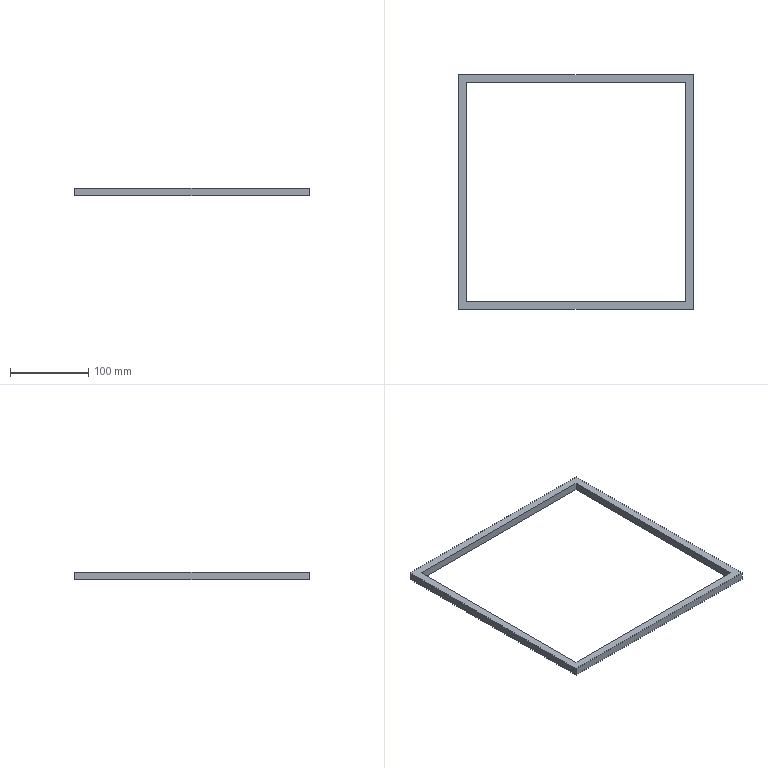Part | SolidWorks | features Extrusion 1 | 1 solid | 10 faces | box 300 x 300 x 10 mm | volume 116000 mm3 | plane 10
STEP:
#1=CARTESIAN_POINT('',(-150.,150.,5.));
#2=VERTEX_POINT('',#1);
#3=CARTESIAN_POINT('',(-150.,-150.,5.));
#4=VERTEX_POINT('',#3);
#5=CARTESIAN_POINT('',(-150.,150.,5.));
#6=DIRECTION('',(0.,-1.,0.));
#7=VECTOR('',#6,1000.);
#8=LINE('',#5,#7);
#9=EDGE_CURVE('',#2,#4,#8,.T.);
#10=ORIENTED_EDGE('',*,*,#9,.F.);
#11=CARTESIAN_POINT('',(-150.,150.,-5.));
#12=VERTEX_POINT('',#11);
#13=CARTESIAN_POINT('',(-150.,150.,-5.));
#14=DIRECTION('',(0.,0.,1.));
#15=VECTOR('',#14,1000.);
#16=LINE('',#13,#15);
#17=EDGE_CURVE('',#12,#2,#16,.T.);
#18=ORIENTED_EDGE('',*,*,#17,.F.);
#19=CARTESIAN_POINT('',(-150.,-150.,-5.));
#20=VERTEX_POINT('',#19);
#21=CARTESIAN_POINT('',(-150.,150.,-5.));
#22=DIRECTION('',(0.,-1.,0.));
#23=VECTOR('',#22,1000.);
#24=LINE('',#21,#23);
#25=EDGE_CURVE('',#12,#20,#24,.T.);
#26=ORIENTED_EDGE('',*,*,#25,.T.);
#27=CARTESIAN_POINT('',(-150.,-150.,-5.));
#28=DIRECTION('',(0.,0.,1.));
#29=VECTOR('',#28,1000.);
#30=LINE('',#27,#29);
#31=EDGE_CURVE('',#20,#4,#30,.T.);
#32=ORIENTED_EDGE('',*,*,#31,.T.);
#33=EDGE_LOOP('',(#10,#18,#26,#32));
#34=FACE_OUTER_BOUND('',#33,.T.);
#35=CARTESIAN_POINT('',(-150.,150.,-5.));
#36=DIRECTION('',(-1.,0.,0.));
#37=DIRECTION('',(0.,0.,1.));
#38=AXIS2_PLACEMENT_3D('',#35,#36,#37);
#39=PLANE('',#38);
#40=ADVANCED_FACE('',(#34),#39,.T.);
#41=CARTESIAN_POINT('',(150.,150.,5.));
#42=VERTEX_POINT('',#41);
#43=CARTESIAN_POINT('',(150.,150.,5.));
#44=DIRECTION('',(-1.,0.,0.));
#45=VECTOR('',#44,1000.);
#46=LINE('',#43,#45);
#47=EDGE_CURVE('',#42,#2,#46,.T.);
#48=ORIENTED_EDGE('',*,*,#47,.F.);
#49=CARTESIAN_POINT('',(150.,150.,-5.));
#50=VERTEX_POINT('',#49);
#51=CARTESIAN_POINT('',(150.,150.,-5.));
#52=DIRECTION('',(0.,0.,1.));
#53=VECTOR('',#52,1000.);
#54=LINE('',#51,#53);
#55=EDGE_CURVE('',#50,#42,#54,.T.);
#56=ORIENTED_EDGE('',*,*,#55,.F.);
#57=CARTESIAN_POINT('',(150.,150.,-5.));
#58=DIRECTION('',(-1.,0.,0.));
#59=VECTOR('',#58,1000.);
#60=LINE('',#57,#59);
#61=EDGE_CURVE('',#50,#12,#60,.T.);
#62=ORIENTED_EDGE('',*,*,#61,.T.);
#63=ORIENTED_EDGE('',*,*,#17,.T.);
#64=EDGE_LOOP('',(#48,#56,#62,#63));
#65=FACE_OUTER_BOUND('',#64,.T.);
#66=CARTESIAN_POINT('',(150.,150.,-5.));
#67=DIRECTION('',(0.,1.,0.));
#68=DIRECTION('',(0.,0.,1.));
#69=AXIS2_PLACEMENT_3D('',#66,#67,#68);
#70=PLANE('',#69);
#71=ADVANCED_FACE('',(#65),#70,.T.);
#72=CARTESIAN_POINT('',(150.,-150.,5.));
#73=VERTEX_POINT('',#72);
#74=CARTESIAN_POINT('',(150.,-150.,5.));
#75=DIRECTION('',(0.,1.,0.));
#76=VECTOR('',#75,1000.);
#77=LINE('',#74,#76);
#78=EDGE_CURVE('',#73,#42,#77,.T.);
#79=ORIENTED_EDGE('',*,*,#78,.F.);
#80=CARTESIAN_POINT('',(150.,-150.,-5.));
#81=VERTEX_POINT('',#80);
#82=CARTESIAN_POINT('',(150.,-150.,-5.));
#83=DIRECTION('',(0.,0.,1.));
#84=VECTOR('',#83,1000.);
#85=LINE('',#82,#84);
#86=EDGE_CURVE('',#81,#73,#85,.T.);
#87=ORIENTED_EDGE('',*,*,#86,.F.);
#88=CARTESIAN_POINT('',(150.,-150.,-5.));
#89=DIRECTION('',(0.,1.,0.));
#90=VECTOR('',#89,1000.);
#91=LINE('',#88,#90);
#92=EDGE_CURVE('',#81,#50,#91,.T.);
#93=ORIENTED_EDGE('',*,*,#92,.T.);
#94=ORIENTED_EDGE('',*,*,#55,.T.);
#95=EDGE_LOOP('',(#79,#87,#93,#94));
#96=FACE_OUTER_BOUND('',#95,.T.);
#97=CARTESIAN_POINT('',(150.,-150.,-5.));
#98=DIRECTION('',(1.,0.,0.));
#99=DIRECTION('',(0.,0.,-1.));
#100=AXIS2_PLACEMENT_3D('',#97,#98,#99);
#101=PLANE('',#100);
#102=ADVANCED_FACE('',(#96),#101,.T.);
#103=CARTESIAN_POINT('',(-150.,-150.,5.));
#104=DIRECTION('',(1.,0.,0.));
#105=VECTOR('',#104,1000.);
#106=LINE('',#103,#105);
#107=EDGE_CURVE('',#4,#73,#106,.T.);
#108=ORIENTED_EDGE('',*,*,#107,.F.);
#109=ORIENTED_EDGE('',*,*,#31,.F.);
#110=CARTESIAN_POINT('',(-150.,-150.,-5.));
#111=DIRECTION('',(1.,0.,0.));
#112=VECTOR('',#111,1000.);
#113=LINE('',#110,#112);
#114=EDGE_CURVE('',#20,#81,#113,.T.);
#115=ORIENTED_EDGE('',*,*,#114,.T.);
#116=ORIENTED_EDGE('',*,*,#86,.T.);
#117=EDGE_LOOP('',(#108,#109,#115,#116));
#118=FACE_OUTER_BOUND('',#117,.T.);
#119=CARTESIAN_POINT('',(-150.,-150.,-5.));
#120=DIRECTION('',(0.,-1.,0.));
#121=DIRECTION('',(0.,0.,-1.));
#122=AXIS2_PLACEMENT_3D('',#119,#120,#121);
#123=PLANE('',#122);
#124=ADVANCED_FACE('',(#118),#123,.T.);
#125=CARTESIAN_POINT('',(140.,140.,-5.));
#126=VERTEX_POINT('',#125);
#127=CARTESIAN_POINT('',(-140.,140.,-5.));
#128=VERTEX_POINT('',#127);
#129=CARTESIAN_POINT('',(140.,140.,-5.));
#130=DIRECTION('',(-1.,0.,0.));
#131=VECTOR('',#130,1000.);
#132=LINE('',#129,#131);
#133=EDGE_CURVE('',#126,#128,#132,.T.);
#134=ORIENTED_EDGE('',*,*,#133,.T.);
#135=CARTESIAN_POINT('',(-140.,-140.,-5.));
#136=VERTEX_POINT('',#135);
#137=CARTESIAN_POINT('',(-140.,140.,-5.));
#138=DIRECTION('',(0.,-1.,0.));
#139=VECTOR('',#138,1000.);
#140=LINE('',#137,#139);
#141=EDGE_CURVE('',#128,#136,#140,.T.);
#142=ORIENTED_EDGE('',*,*,#141,.T.);
#143=CARTESIAN_POINT('',(140.,-140.,-5.));
#144=VERTEX_POINT('',#143);
#145=CARTESIAN_POINT('',(-140.,-140.,-5.));
#146=DIRECTION('',(1.,0.,0.));
#147=VECTOR('',#146,1000.);
#148=LINE('',#145,#147);
#149=EDGE_CURVE('',#136,#144,#148,.T.);
#150=ORIENTED_EDGE('',*,*,#149,.T.);
#151=CARTESIAN_POINT('',(140.,-140.,-5.));
#152=DIRECTION('',(0.,1.,0.));
#153=VECTOR('',#152,1000.);
#154=LINE('',#151,#153);
#155=EDGE_CURVE('',#144,#126,#154,.T.);
#156=ORIENTED_EDGE('',*,*,#155,.T.);
#157=EDGE_LOOP('',(#134,#142,#150,#156));
#158=FACE_BOUND('',#157,.T.);
#159=ORIENTED_EDGE('',*,*,#25,.F.);
#160=ORIENTED_EDGE('',*,*,#61,.F.);
#161=ORIENTED_EDGE('',*,*,#92,.F.);
#162=ORIENTED_EDGE('',*,*,#114,.F.);
#163=EDGE_LOOP('',(#159,#160,#161,#162));
#164=FACE_OUTER_BOUND('',#163,.T.);
#165=CARTESIAN_POINT('',(0.,0.,-5.));
#166=DIRECTION('',(0.,0.,1.));
#167=DIRECTION('',(1.,0.,0.));
#168=AXIS2_PLACEMENT_3D('',#165,#166,#167);
#169=PLANE('',#168);
#170=ADVANCED_FACE('',(#158,#164),#169,.F.);
#171=CARTESIAN_POINT('',(-140.,140.,5.));
#172=VERTEX_POINT('',#171);
#173=CARTESIAN_POINT('',(-140.,-140.,5.));
#174=VERTEX_POINT('',#173);
#175=CARTESIAN_POINT('',(-140.,140.,5.));
#176=DIRECTION('',(0.,-1.,0.));
#177=VECTOR('',#176,1000.);
#178=LINE('',#175,#177);
#179=EDGE_CURVE('',#172,#174,#178,.T.);
#180=ORIENTED_EDGE('',*,*,#179,.F.);
#181=CARTESIAN_POINT('',(140.,140.,5.));
#182=VERTEX_POINT('',#181);
#183=CARTESIAN_POINT('',(140.,140.,5.));
#184=DIRECTION('',(-1.,0.,0.));
#185=VECTOR('',#184,1000.);
#186=LINE('',#183,#185);
#187=EDGE_CURVE('',#182,#172,#186,.T.);
#188=ORIENTED_EDGE('',*,*,#187,.F.);
#189=CARTESIAN_POINT('',(140.,-140.,5.));
#190=VERTEX_POINT('',#189);
#191=CARTESIAN_POINT('',(140.,-140.,5.));
#192=DIRECTION('',(0.,1.,0.));
#193=VECTOR('',#192,1000.);
#194=LINE('',#191,#193);
#195=EDGE_CURVE('',#190,#182,#194,.T.);
#196=ORIENTED_EDGE('',*,*,#195,.F.);
#197=CARTESIAN_POINT('',(-140.,-140.,5.));
#198=DIRECTION('',(1.,0.,0.));
#199=VECTOR('',#198,1000.);
#200=LINE('',#197,#199);
#201=EDGE_CURVE('',#174,#190,#200,.T.);
#202=ORIENTED_EDGE('',*,*,#201,.F.);
#203=EDGE_LOOP('',(#180,#188,#196,#202));
#204=FACE_BOUND('',#203,.T.);
#205=ORIENTED_EDGE('',*,*,#9,.T.);
#206=ORIENTED_EDGE('',*,*,#107,.T.);
#207=ORIENTED_EDGE('',*,*,#78,.T.);
#208=ORIENTED_EDGE('',*,*,#47,.T.);
#209=EDGE_LOOP('',(#205,#206,#207,#208));
#210=FACE_OUTER_BOUND('',#209,.T.);
#211=CARTESIAN_POINT('',(0.,0.,5.));
#212=DIRECTION('',(0.,0.,1.));
#213=DIRECTION('',(1.,0.,0.));
#214=AXIS2_PLACEMENT_3D('',#211,#212,#213);
#215=PLANE('',#214);
#216=ADVANCED_FACE('',(#204,#210),#215,.T.);
#217=ORIENTED_EDGE('',*,*,#179,.T.);
#218=CARTESIAN_POINT('',(-140.,-140.,-5.));
#219=DIRECTION('',(0.,0.,1.));
#220=VECTOR('',#219,1000.);
#221=LINE('',#218,#220);
#222=EDGE_CURVE('',#136,#174,#221,.T.);
#223=ORIENTED_EDGE('',*,*,#222,.F.);
#224=ORIENTED_EDGE('',*,*,#141,.F.);
#225=CARTESIAN_POINT('',(-140.,140.,-5.));
#226=DIRECTION('',(0.,0.,1.));
#227=VECTOR('',#226,1000.);
#228=LINE('',#225,#227);
#229=EDGE_CURVE('',#128,#172,#228,.T.);
#230=ORIENTED_EDGE('',*,*,#229,.T.);
#231=EDGE_LOOP('',(#217,#223,#224,#230));
#232=FACE_OUTER_BOUND('',#231,.T.);
#233=CARTESIAN_POINT('',(-140.,140.,-5.));
#234=DIRECTION('',(-1.,0.,0.));
#235=DIRECTION('',(0.,0.,1.));
#236=AXIS2_PLACEMENT_3D('',#233,#234,#235);
#237=PLANE('',#236);
#238=ADVANCED_FACE('',(#232),#237,.F.);
#239=ORIENTED_EDGE('',*,*,#187,.T.);
#240=ORIENTED_EDGE('',*,*,#229,.F.);
#241=ORIENTED_EDGE('',*,*,#133,.F.);
#242=CARTESIAN_POINT('',(140.,140.,-5.));
#243=DIRECTION('',(0.,0.,1.));
#244=VECTOR('',#243,1000.);
#245=LINE('',#242,#244);
#246=EDGE_CURVE('',#126,#182,#245,.T.);
#247=ORIENTED_EDGE('',*,*,#246,.T.);
#248=EDGE_LOOP('',(#239,#240,#241,#247));
#249=FACE_OUTER_BOUND('',#248,.T.);
#250=CARTESIAN_POINT('',(140.,140.,-5.));
#251=DIRECTION('',(0.,1.,0.));
#252=DIRECTION('',(0.,0.,1.));
#253=AXIS2_PLACEMENT_3D('',#250,#251,#252);
#254=PLANE('',#253);
#255=ADVANCED_FACE('',(#249),#254,.F.);
#256=ORIENTED_EDGE('',*,*,#195,.T.);
#257=ORIENTED_EDGE('',*,*,#246,.F.);
#258=ORIENTED_EDGE('',*,*,#155,.F.);
#259=CARTESIAN_POINT('',(140.,-140.,-5.));
#260=DIRECTION('',(0.,0.,1.));
#261=VECTOR('',#260,1000.);
#262=LINE('',#259,#261);
#263=EDGE_CURVE('',#144,#190,#262,.T.);
#264=ORIENTED_EDGE('',*,*,#263,.T.);
#265=EDGE_LOOP('',(#256,#257,#258,#264));
#266=FACE_OUTER_BOUND('',#265,.T.);
#267=CARTESIAN_POINT('',(140.,-140.,-5.));
#268=DIRECTION('',(1.,0.,0.));
#269=DIRECTION('',(0.,0.,-1.));
#270=AXIS2_PLACEMENT_3D('',#267,#268,#269);
#271=PLANE('',#270);
#272=ADVANCED_FACE('',(#266),#271,.F.);
#273=ORIENTED_EDGE('',*,*,#201,.T.);
#274=ORIENTED_EDGE('',*,*,#263,.F.);
#275=ORIENTED_EDGE('',*,*,#149,.F.);
#276=ORIENTED_EDGE('',*,*,#222,.T.);
#277=EDGE_LOOP('',(#273,#274,#275,#276));
#278=FACE_OUTER_BOUND('',#277,.T.);
#279=CARTESIAN_POINT('',(-140.,-140.,-5.));
#280=DIRECTION('',(0.,-1.,0.));
#281=DIRECTION('',(0.,0.,-1.));
#282=AXIS2_PLACEMENT_3D('',#279,#280,#281);
#283=PLANE('',#282);
#284=ADVANCED_FACE('',(#278),#283,.F.);
#285=CLOSED_SHELL('',(#40,#71,#102,#124,#170,#216,#238,#255,#272,#284));
#286=MANIFOLD_SOLID_BREP('',#285);
#287=CARTESIAN_POINT('',(0.,0.,0.));
#288=DIRECTION('',(0.,0.,1.));
#289=DIRECTION('',(1.,0.,0.));
#290=AXIS2_PLACEMENT_3D('',#287,#288,#289);
#291=(LENGTH_UNIT()NAMED_UNIT(*)SI_UNIT(.MILLI.,.METRE.));
#292=UNCERTAINTY_MEASURE_WITH_UNIT(LENGTH_MEASURE(0.00001),#291,'','');
#293=(NAMED_UNIT(*)PLANE_ANGLE_UNIT()SI_UNIT($,.RADIAN.));
#294=(NAMED_UNIT(*)SI_UNIT($,.STERADIAN.)SOLID_ANGLE_UNIT());
#295=(GEOMETRIC_REPRESENTATION_CONTEXT(3)GLOBAL_UNCERTAINTY_ASSIGNED_CONTEXT((#292))GLOBAL_UNIT_ASSIGNED_CONTEXT((#291,#293,#294))REPRESENTATION_CONTEXT('',''));
#296=ADVANCED_BREP_SHAPE_REPRESENTATION('',(#286,#290),#295);